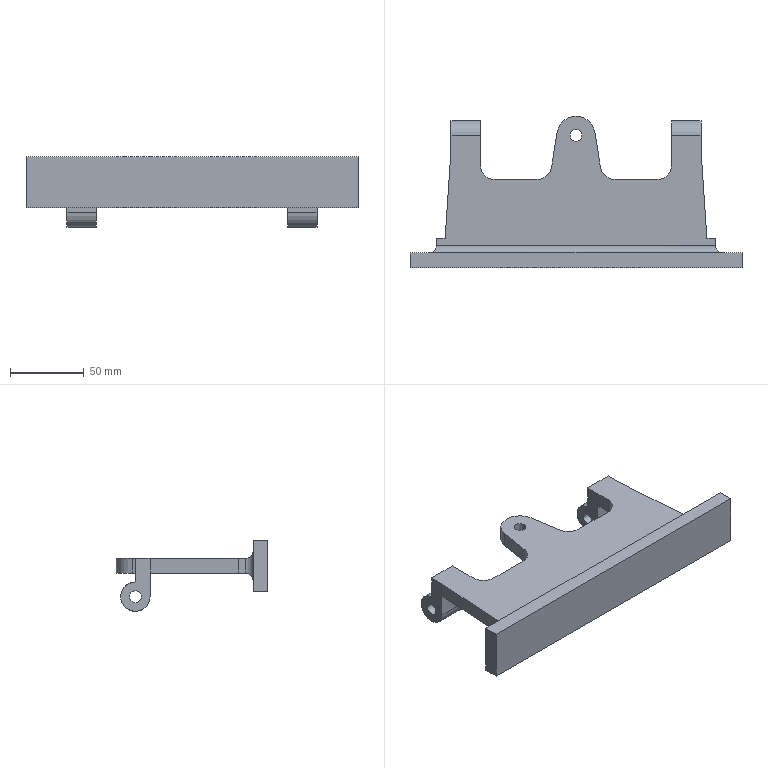Part | SolidWorks | features ICE 2, Extrusion 1, Fillet 1, MirrorPattern 1 | 1 solid | 44 faces | box 225.743 x 103 x 48.082 mm | volume 208388 mm3 | plane 26 | cylinder 18 | commonest cylinder face diameters 20 x7 8 x6 10 x4 26 x1
STEP:
#1=CARTESIAN_POINT('',(85.,-4.,-16.));
#2=VERTEX_POINT('',#1);
#3=CARTESIAN_POINT('',(85.,4.,-16.));
#4=VERTEX_POINT('',#3);
#5=CARTESIAN_POINT('',(85.,0.,-16.));
#6=DIRECTION('',(1.,0.,0.));
#7=DIRECTION('',(0.,1.,0.));
#8=AXIS2_PLACEMENT_3D('',#5,#6,#7);
#9=CIRCLE('',#8,4.);
#10=EDGE_CURVE('',#2,#4,#9,.T.);
#11=ORIENTED_EDGE('',*,*,#10,.T.);
#12=CARTESIAN_POINT('',(65.,4.,-16.));
#13=VERTEX_POINT('',#12);
#14=CARTESIAN_POINT('',(85.,4.,-16.));
#15=DIRECTION('',(-1.,0.,0.));
#16=VECTOR('',#15,1000.);
#17=LINE('',#14,#16);
#18=EDGE_CURVE('',#4,#13,#17,.T.);
#19=ORIENTED_EDGE('',*,*,#18,.T.);
#20=CARTESIAN_POINT('',(65.,-4.,-16.));
#21=VERTEX_POINT('',#20);
#22=CARTESIAN_POINT('',(65.,0.,-16.));
#23=DIRECTION('',(1.,0.,0.));
#24=DIRECTION('',(0.,1.,0.));
#25=AXIS2_PLACEMENT_3D('',#22,#23,#24);
#26=CIRCLE('',#25,4.);
#27=EDGE_CURVE('',#21,#13,#26,.T.);
#28=ORIENTED_EDGE('',*,*,#27,.F.);
#29=CARTESIAN_POINT('',(85.,-4.,-16.));
#30=DIRECTION('',(-1.,0.,0.));
#31=VECTOR('',#30,1000.);
#32=LINE('',#29,#31);
#33=EDGE_CURVE('',#2,#21,#32,.T.);
#34=ORIENTED_EDGE('',*,*,#33,.F.);
#35=EDGE_LOOP('',(#11,#19,#28,#34));
#36=FACE_OUTER_BOUND('',#35,.T.);
#37=CARTESIAN_POINT('',(85.,0.,-16.));
#38=DIRECTION('',(-1.,0.,0.));
#39=DIRECTION('',(0.,-1.,0.));
#40=AXIS2_PLACEMENT_3D('',#37,#38,#39);
#41=CYLINDRICAL_SURFACE('',#40,4.);
#42=ADVANCED_FACE('',(#36),#41,.F.);
#43=CARTESIAN_POINT('',(-85.,-4.,-16.));
#44=VERTEX_POINT('',#43);
#45=CARTESIAN_POINT('',(-85.,4.,-16.));
#46=VERTEX_POINT('',#45);
#47=CARTESIAN_POINT('',(-85.,0.,-16.));
#48=DIRECTION('',(1.,0.,0.));
#49=DIRECTION('',(0.,1.,0.));
#50=AXIS2_PLACEMENT_3D('',#47,#48,#49);
#51=CIRCLE('',#50,4.);
#52=EDGE_CURVE('',#44,#46,#51,.T.);
#53=ORIENTED_EDGE('',*,*,#52,.F.);
#54=CARTESIAN_POINT('',(-65.,-4.,-16.));
#55=VERTEX_POINT('',#54);
#56=CARTESIAN_POINT('',(-85.,-4.,-16.));
#57=DIRECTION('',(1.,0.,0.));
#58=VECTOR('',#57,1000.);
#59=LINE('',#56,#58);
#60=EDGE_CURVE('',#44,#55,#59,.T.);
#61=ORIENTED_EDGE('',*,*,#60,.T.);
#62=CARTESIAN_POINT('',(-65.,4.,-16.));
#63=VERTEX_POINT('',#62);
#64=CARTESIAN_POINT('',(-65.,0.,-16.));
#65=DIRECTION('',(1.,0.,0.));
#66=DIRECTION('',(0.,1.,0.));
#67=AXIS2_PLACEMENT_3D('',#64,#65,#66);
#68=CIRCLE('',#67,4.);
#69=EDGE_CURVE('',#55,#63,#68,.T.);
#70=ORIENTED_EDGE('',*,*,#69,.T.);
#71=CARTESIAN_POINT('',(-85.,4.,-16.));
#72=DIRECTION('',(1.,0.,0.));
#73=VECTOR('',#72,1000.);
#74=LINE('',#71,#73);
#75=EDGE_CURVE('',#46,#63,#74,.T.);
#76=ORIENTED_EDGE('',*,*,#75,.F.);
#77=EDGE_LOOP('',(#53,#61,#70,#76));
#78=FACE_OUTER_BOUND('',#77,.T.);
#79=CARTESIAN_POINT('',(-85.,0.,-16.));
#80=DIRECTION('',(1.,0.,0.));
#81=DIRECTION('',(0.,1.,0.));
#82=AXIS2_PLACEMENT_3D('',#79,#80,#81);
#83=CYLINDRICAL_SURFACE('',#82,4.);
#84=ADVANCED_FACE('',(#78),#83,.F.);
#85=CARTESIAN_POINT('',(-85.,-10.,-16.));
#86=VERTEX_POINT('',#85);
#87=CARTESIAN_POINT('',(-85.,10.,-16.));
#88=VERTEX_POINT('',#87);
#89=CARTESIAN_POINT('',(-85.,0.,-16.));
#90=DIRECTION('',(1.,0.,0.));
#91=DIRECTION('',(0.,1.,0.));
#92=AXIS2_PLACEMENT_3D('',#89,#90,#91);
#93=CIRCLE('',#92,10.);
#94=EDGE_CURVE('',#86,#88,#93,.T.);
#95=ORIENTED_EDGE('',*,*,#94,.T.);
#96=CARTESIAN_POINT('',(-65.,10.,-16.));
#97=VERTEX_POINT('',#96);
#98=CARTESIAN_POINT('',(-85.,10.,-16.));
#99=DIRECTION('',(1.,0.,0.));
#100=VECTOR('',#99,1000.);
#101=LINE('',#98,#100);
#102=EDGE_CURVE('',#88,#97,#101,.T.);
#103=ORIENTED_EDGE('',*,*,#102,.T.);
#104=CARTESIAN_POINT('',(-65.,-10.,-16.));
#105=VERTEX_POINT('',#104);
#106=CARTESIAN_POINT('',(-65.,0.,-16.));
#107=DIRECTION('',(1.,0.,0.));
#108=DIRECTION('',(0.,1.,0.));
#109=AXIS2_PLACEMENT_3D('',#106,#107,#108);
#110=CIRCLE('',#109,10.);
#111=EDGE_CURVE('',#105,#97,#110,.T.);
#112=ORIENTED_EDGE('',*,*,#111,.F.);
#113=CARTESIAN_POINT('',(-85.,-10.,-16.));
#114=DIRECTION('',(1.,0.,0.));
#115=VECTOR('',#114,1000.);
#116=LINE('',#113,#115);
#117=EDGE_CURVE('',#86,#105,#116,.T.);
#118=ORIENTED_EDGE('',*,*,#117,.F.);
#119=EDGE_LOOP('',(#95,#103,#112,#118));
#120=FACE_OUTER_BOUND('',#119,.T.);
#121=CARTESIAN_POINT('',(-85.,0.,-16.));
#122=DIRECTION('',(1.,0.,0.));
#123=DIRECTION('',(0.,1.,0.));
#124=AXIS2_PLACEMENT_3D('',#121,#122,#123);
#125=CYLINDRICAL_SURFACE('',#124,10.);
#126=ADVANCED_FACE('',(#120),#125,.T.);
#127=CARTESIAN_POINT('',(-4.,0.,10.));
#128=VERTEX_POINT('',#127);
#129=CARTESIAN_POINT('',(4.,0.,10.));
#130=VERTEX_POINT('',#129);
#131=CARTESIAN_POINT('',(0.,0.,10.));
#132=DIRECTION('',(0.,0.,1.));
#133=DIRECTION('',(1.,0.,0.));
#134=AXIS2_PLACEMENT_3D('',#131,#132,#133);
#135=CIRCLE('',#134,4.);
#136=EDGE_CURVE('',#128,#130,#135,.T.);
#137=ORIENTED_EDGE('',*,*,#136,.T.);
#138=CARTESIAN_POINT('',(4.,0.,0.));
#139=VERTEX_POINT('',#138);
#140=CARTESIAN_POINT('',(4.,0.,10.));
#141=DIRECTION('',(0.,0.,-1.));
#142=VECTOR('',#141,1000.);
#143=LINE('',#140,#142);
#144=EDGE_CURVE('',#130,#139,#143,.T.);
#145=ORIENTED_EDGE('',*,*,#144,.T.);
#146=CARTESIAN_POINT('',(-4.,0.,0.));
#147=VERTEX_POINT('',#146);
#148=CARTESIAN_POINT('',(0.,0.,0.));
#149=DIRECTION('',(0.,0.,1.));
#150=DIRECTION('',(1.,0.,0.));
#151=AXIS2_PLACEMENT_3D('',#148,#149,#150);
#152=CIRCLE('',#151,4.);
#153=EDGE_CURVE('',#147,#139,#152,.T.);
#154=ORIENTED_EDGE('',*,*,#153,.F.);
#155=CARTESIAN_POINT('',(-4.,0.,10.));
#156=DIRECTION('',(0.,0.,-1.));
#157=VECTOR('',#156,1000.);
#158=LINE('',#155,#157);
#159=EDGE_CURVE('',#128,#147,#158,.T.);
#160=ORIENTED_EDGE('',*,*,#159,.F.);
#161=EDGE_LOOP('',(#137,#145,#154,#160));
#162=FACE_OUTER_BOUND('',#161,.T.);
#163=CARTESIAN_POINT('',(0.,0.,10.));
#164=DIRECTION('',(0.,0.,-1.));
#165=DIRECTION('',(-1.,0.,0.));
#166=AXIS2_PLACEMENT_3D('',#163,#164,#165);
#167=CYLINDRICAL_SURFACE('',#166,4.);
#168=ADVANCED_FACE('',(#162),#167,.F.);
#169=CARTESIAN_POINT('',(-95.,-70.,10.));
#170=VERTEX_POINT('',#169);
#171=CARTESIAN_POINT('',(-95.,-75.,10.));
#172=VERTEX_POINT('',#171);
#173=CARTESIAN_POINT('',(-95.,-80.,10.));
#174=DIRECTION('',(0.,-1.,0.));
#175=VECTOR('',#174,1000.);
#176=LINE('',#173,#175);
#177=EDGE_CURVE('',#170,#172,#176,.T.);
#178=ORIENTED_EDGE('',*,*,#177,.T.);
#179=CARTESIAN_POINT('',(95.,-75.,10.));
#180=VERTEX_POINT('',#179);
#181=CARTESIAN_POINT('',(95.,-75.,10.));
#182=DIRECTION('',(1.,0.,0.));
#183=VECTOR('',#182,1000.);
#184=LINE('',#181,#183);
#185=EDGE_CURVE('',#172,#180,#184,.T.);
#186=ORIENTED_EDGE('',*,*,#185,.T.);
#187=CARTESIAN_POINT('',(95.,-70.,10.));
#188=VERTEX_POINT('',#187);
#189=CARTESIAN_POINT('',(95.,-80.,10.));
#190=DIRECTION('',(0.,1.,0.));
#191=VECTOR('',#190,1000.);
#192=LINE('',#189,#191);
#193=EDGE_CURVE('',#180,#188,#192,.T.);
#194=ORIENTED_EDGE('',*,*,#193,.T.);
#195=CARTESIAN_POINT('',(89.,-70.,10.));
#196=VERTEX_POINT('',#195);
#197=CARTESIAN_POINT('',(95.,-70.,10.));
#198=DIRECTION('',(-1.,0.,0.));
#199=VECTOR('',#198,1000.);
#200=LINE('',#197,#199);
#201=EDGE_CURVE('',#188,#196,#200,.T.);
#202=ORIENTED_EDGE('',*,*,#201,.T.);
#203=CARTESIAN_POINT('',(85.,-10.,10.));
#204=VERTEX_POINT('',#203);
#205=CARTESIAN_POINT('',(85.,-10.,10.));
#206=DIRECTION('',(-0.06652,0.9978,0.));
#207=VECTOR('',#206,1000.);
#208=LINE('',#205,#207);
#209=EDGE_CURVE('',#196,#204,#208,.T.);
#210=ORIENTED_EDGE('',*,*,#209,.T.);
#211=CARTESIAN_POINT('',(85.,0.,10.));
#212=VERTEX_POINT('',#211);
#213=CARTESIAN_POINT('',(85.,0.,10.));
#214=DIRECTION('',(0.,-1.,0.));
#215=VECTOR('',#214,1000.);
#216=LINE('',#213,#215);
#217=EDGE_CURVE('',#212,#204,#216,.T.);
#218=ORIENTED_EDGE('',*,*,#217,.F.);
#219=CARTESIAN_POINT('',(65.,0.,10.));
#220=VERTEX_POINT('',#219);
#221=CARTESIAN_POINT('',(85.,0.,10.));
#222=DIRECTION('',(-1.,0.,0.));
#223=VECTOR('',#222,1000.);
#224=LINE('',#221,#223);
#225=EDGE_CURVE('',#212,#220,#224,.T.);
#226=ORIENTED_EDGE('',*,*,#225,.T.);
#227=CARTESIAN_POINT('',(65.,-20.,10.));
#228=VERTEX_POINT('',#227);
#229=CARTESIAN_POINT('',(65.,-10.,10.));
#230=DIRECTION('',(0.,-1.,0.));
#231=VECTOR('',#230,1000.);
#232=LINE('',#229,#231);
#233=EDGE_CURVE('',#220,#228,#232,.T.);
#234=ORIENTED_EDGE('',*,*,#233,.T.);
#235=CARTESIAN_POINT('',(55.,-30.,10.));
#236=VERTEX_POINT('',#235);
#237=CARTESIAN_POINT('',(55.,-20.,10.));
#238=DIRECTION('',(0.,0.,-1.));
#239=DIRECTION('',(-1.,0.,0.));
#240=AXIS2_PLACEMENT_3D('',#237,#238,#239);
#241=CIRCLE('',#240,10.);
#242=EDGE_CURVE('',#228,#236,#241,.T.);
#243=ORIENTED_EDGE('',*,*,#242,.T.);
#244=CARTESIAN_POINT('',(26.518,-30.,10.));
#245=VERTEX_POINT('',#244);
#246=CARTESIAN_POINT('',(26.518,-30.,10.));
#247=DIRECTION('',(-1.,0.,0.));
#248=VECTOR('',#247,1000.);
#249=LINE('',#246,#248);
#250=EDGE_CURVE('',#236,#245,#249,.T.);
#251=ORIENTED_EDGE('',*,*,#250,.T.);
#252=CARTESIAN_POINT('',(16.645,-21.59,10.));
#253=VERTEX_POINT('',#252);
#254=CARTESIAN_POINT('',(26.518,-20.,10.));
#255=DIRECTION('',(0.,0.,-1.));
#256=DIRECTION('',(1.,0.,0.));
#257=AXIS2_PLACEMENT_3D('',#254,#255,#256);
#258=CIRCLE('',#257,10.);
#259=EDGE_CURVE('',#245,#253,#258,.T.);
#260=ORIENTED_EDGE('',*,*,#259,.T.);
#261=CARTESIAN_POINT('',(12.835,2.067,10.));
#262=VERTEX_POINT('',#261);
#263=CARTESIAN_POINT('',(12.835,2.067,10.));
#264=DIRECTION('',(-0.159,0.9873,0.));
#265=VECTOR('',#264,1000.);
#266=LINE('',#263,#265);
#267=EDGE_CURVE('',#253,#262,#266,.T.);
#268=ORIENTED_EDGE('',*,*,#267,.T.);
#269=CARTESIAN_POINT('',(-12.835,2.067,10.));
#270=VERTEX_POINT('',#269);
#271=CARTESIAN_POINT('',(0.,0.,10.));
#272=DIRECTION('',(0.,0.,1.));
#273=DIRECTION('',(1.,0.,0.));
#274=AXIS2_PLACEMENT_3D('',#271,#272,#273);
#275=CIRCLE('',#274,13.);
#276=EDGE_CURVE('',#262,#270,#275,.T.);
#277=ORIENTED_EDGE('',*,*,#276,.T.);
#278=CARTESIAN_POINT('',(-16.645,-21.59,10.));
#279=VERTEX_POINT('',#278);
#280=CARTESIAN_POINT('',(-12.835,2.067,10.));
#281=DIRECTION('',(-0.159,-0.9873,0.));
#282=VECTOR('',#281,1000.);
#283=LINE('',#280,#282);
#284=EDGE_CURVE('',#270,#279,#283,.T.);
#285=ORIENTED_EDGE('',*,*,#284,.T.);
#286=CARTESIAN_POINT('',(-26.518,-30.,10.));
#287=VERTEX_POINT('',#286);
#288=CARTESIAN_POINT('',(-26.518,-20.,10.));
#289=DIRECTION('',(0.,0.,-1.));
#290=DIRECTION('',(-1.,0.,0.));
#291=AXIS2_PLACEMENT_3D('',#288,#289,#290);
#292=CIRCLE('',#291,10.);
#293=EDGE_CURVE('',#279,#287,#292,.T.);
#294=ORIENTED_EDGE('',*,*,#293,.T.);
#295=CARTESIAN_POINT('',(-55.,-30.,10.));
#296=VERTEX_POINT('',#295);
#297=CARTESIAN_POINT('',(-55.,-30.,10.));
#298=DIRECTION('',(-1.,0.,0.));
#299=VECTOR('',#298,1000.);
#300=LINE('',#297,#299);
#301=EDGE_CURVE('',#287,#296,#300,.T.);
#302=ORIENTED_EDGE('',*,*,#301,.T.);
#303=CARTESIAN_POINT('',(-65.,-20.,10.));
#304=VERTEX_POINT('',#303);
#305=CARTESIAN_POINT('',(-55.,-20.,10.));
#306=DIRECTION('',(0.,0.,-1.));
#307=DIRECTION('',(1.,0.,0.));
#308=AXIS2_PLACEMENT_3D('',#305,#306,#307);
#309=CIRCLE('',#308,10.);
#310=EDGE_CURVE('',#296,#304,#309,.T.);
#311=ORIENTED_EDGE('',*,*,#310,.T.);
#312=CARTESIAN_POINT('',(-65.,0.,10.));
#313=VERTEX_POINT('',#312);
#314=CARTESIAN_POINT('',(-65.,-10.,10.));
#315=DIRECTION('',(0.,1.,0.));
#316=VECTOR('',#315,1000.);
#317=LINE('',#314,#316);
#318=EDGE_CURVE('',#304,#313,#317,.T.);
#319=ORIENTED_EDGE('',*,*,#318,.T.);
#320=CARTESIAN_POINT('',(-85.,0.,10.));
#321=VERTEX_POINT('',#320);
#322=CARTESIAN_POINT('',(-85.,0.,10.));
#323=DIRECTION('',(1.,0.,0.));
#324=VECTOR('',#323,1000.);
#325=LINE('',#322,#324);
#326=EDGE_CURVE('',#321,#313,#325,.T.);
#327=ORIENTED_EDGE('',*,*,#326,.F.);
#328=CARTESIAN_POINT('',(-85.,-10.,10.));
#329=VERTEX_POINT('',#328);
#330=CARTESIAN_POINT('',(-85.,0.,10.));
#331=DIRECTION('',(0.,-1.,0.));
#332=VECTOR('',#331,1000.);
#333=LINE('',#330,#332);
#334=EDGE_CURVE('',#321,#329,#333,.T.);
#335=ORIENTED_EDGE('',*,*,#334,.T.);
#336=CARTESIAN_POINT('',(-89.,-70.,10.));
#337=VERTEX_POINT('',#336);
#338=CARTESIAN_POINT('',(-85.,-10.,10.));
#339=DIRECTION('',(-0.06652,-0.9978,0.));
#340=VECTOR('',#339,1000.);
#341=LINE('',#338,#340);
#342=EDGE_CURVE('',#329,#337,#341,.T.);
#343=ORIENTED_EDGE('',*,*,#342,.T.);
#344=CARTESIAN_POINT('',(-95.,-70.,10.));
#345=DIRECTION('',(-1.,0.,0.));
#346=VECTOR('',#345,1000.);
#347=LINE('',#344,#346);
#348=EDGE_CURVE('',#337,#170,#347,.T.);
#349=ORIENTED_EDGE('',*,*,#348,.T.);
#350=EDGE_LOOP('',(#178,#186,#194,#202,#210,#218,#226,#234,#243,#251,#260,#268,#277,#285,#294,#302,#311,#319,#327,#335,#343,#349));
#351=FACE_OUTER_BOUND('',#350,.T.);
#352=ORIENTED_EDGE('',*,*,#136,.F.);
#353=CARTESIAN_POINT('',(0.,0.,10.));
#354=DIRECTION('',(0.,0.,1.));
#355=DIRECTION('',(1.,0.,0.));
#356=AXIS2_PLACEMENT_3D('',#353,#354,#355);
#357=CIRCLE('',#356,4.);
#358=EDGE_CURVE('',#130,#128,#357,.T.);
#359=ORIENTED_EDGE('',*,*,#358,.F.);
#360=EDGE_LOOP('',(#352,#359));
#361=FACE_BOUND('',#360,.T.);
#362=CARTESIAN_POINT('',(55.,-20.,10.));
#363=DIRECTION('',(0.,0.,-1.));
#364=DIRECTION('',(-1.,0.,0.));
#365=AXIS2_PLACEMENT_3D('',#362,#363,#364);
#366=PLANE('',#365);
#367=ADVANCED_FACE('',(#351,#361),#366,.F.);
#368=CARTESIAN_POINT('',(95.,-75.,0.));
#369=VERTEX_POINT('',#368);
#370=CARTESIAN_POINT('',(95.,-70.,0.));
#371=VERTEX_POINT('',#370);
#372=CARTESIAN_POINT('',(95.,-80.,0.));
#373=DIRECTION('',(0.,1.,0.));
#374=VECTOR('',#373,1000.);
#375=LINE('',#372,#374);
#376=EDGE_CURVE('',#369,#371,#375,.T.);
#377=ORIENTED_EDGE('',*,*,#376,.F.);
#378=CARTESIAN_POINT('',(-95.,-75.,0.));
#379=VERTEX_POINT('',#378);
#380=CARTESIAN_POINT('',(55.,-75.,0.));
#381=DIRECTION('',(-1.,0.,0.));
#382=VECTOR('',#381,1000.);
#383=LINE('',#380,#382);
#384=EDGE_CURVE('',#369,#379,#383,.T.);
#385=ORIENTED_EDGE('',*,*,#384,.T.);
#386=CARTESIAN_POINT('',(-95.,-70.,0.));
#387=VERTEX_POINT('',#386);
#388=CARTESIAN_POINT('',(-95.,-80.,0.));
#389=DIRECTION('',(0.,-1.,0.));
#390=VECTOR('',#389,1000.);
#391=LINE('',#388,#390);
#392=EDGE_CURVE('',#387,#379,#391,.T.);
#393=ORIENTED_EDGE('',*,*,#392,.F.);
#394=CARTESIAN_POINT('',(-89.,-70.,0.));
#395=VERTEX_POINT('',#394);
#396=CARTESIAN_POINT('',(-95.,-70.,0.));
#397=DIRECTION('',(-1.,0.,0.));
#398=VECTOR('',#397,1000.);
#399=LINE('',#396,#398);
#400=EDGE_CURVE('',#395,#387,#399,.T.);
#401=ORIENTED_EDGE('',*,*,#400,.F.);
#402=CARTESIAN_POINT('',(-85.,-10.,0.));
#403=VERTEX_POINT('',#402);
#404=CARTESIAN_POINT('',(-85.,-10.,0.));
#405=DIRECTION('',(-0.06652,-0.9978,0.));
#406=VECTOR('',#405,1000.);
#407=LINE('',#404,#406);
#408=EDGE_CURVE('',#403,#395,#407,.T.);
#409=ORIENTED_EDGE('',*,*,#408,.F.);
#410=CARTESIAN_POINT('',(-65.,-10.,0.));
#411=VERTEX_POINT('',#410);
#412=CARTESIAN_POINT('',(-65.,-10.,0.));
#413=DIRECTION('',(-1.,0.,0.));
#414=VECTOR('',#413,1000.);
#415=LINE('',#412,#414);
#416=EDGE_CURVE('',#411,#403,#415,.T.);
#417=ORIENTED_EDGE('',*,*,#416,.F.);
#418=CARTESIAN_POINT('',(-65.,-20.,0.));
#419=VERTEX_POINT('',#418);
#420=CARTESIAN_POINT('',(-65.,-10.,0.));
#421=DIRECTION('',(0.,1.,0.));
#422=VECTOR('',#421,1000.);
#423=LINE('',#420,#422);
#424=EDGE_CURVE('',#419,#411,#423,.T.);
#425=ORIENTED_EDGE('',*,*,#424,.F.);
#426=CARTESIAN_POINT('',(-55.,-30.,0.));
#427=VERTEX_POINT('',#426);
#428=CARTESIAN_POINT('',(-55.,-20.,0.));
#429=DIRECTION('',(0.,0.,-1.));
#430=DIRECTION('',(1.,0.,0.));
#431=AXIS2_PLACEMENT_3D('',#428,#429,#430);
#432=CIRCLE('',#431,10.);
#433=EDGE_CURVE('',#427,#419,#432,.T.);
#434=ORIENTED_EDGE('',*,*,#433,.F.);
#435=CARTESIAN_POINT('',(-26.518,-30.,0.));
#436=VERTEX_POINT('',#435);
#437=CARTESIAN_POINT('',(-55.,-30.,0.));
#438=DIRECTION('',(-1.,0.,0.));
#439=VECTOR('',#438,1000.);
#440=LINE('',#437,#439);
#441=EDGE_CURVE('',#436,#427,#440,.T.);
#442=ORIENTED_EDGE('',*,*,#441,.F.);
#443=CARTESIAN_POINT('',(-16.645,-21.59,0.));
#444=VERTEX_POINT('',#443);
#445=CARTESIAN_POINT('',(-26.518,-20.,0.));
#446=DIRECTION('',(0.,0.,-1.));
#447=DIRECTION('',(-1.,0.,0.));
#448=AXIS2_PLACEMENT_3D('',#445,#446,#447);
#449=CIRCLE('',#448,10.);
#450=EDGE_CURVE('',#444,#436,#449,.T.);
#451=ORIENTED_EDGE('',*,*,#450,.F.);
#452=CARTESIAN_POINT('',(-12.835,2.067,0.));
#453=VERTEX_POINT('',#452);
#454=CARTESIAN_POINT('',(-12.835,2.067,0.));
#455=DIRECTION('',(-0.159,-0.9873,0.));
#456=VECTOR('',#455,1000.);
#457=LINE('',#454,#456);
#458=EDGE_CURVE('',#453,#444,#457,.T.);
#459=ORIENTED_EDGE('',*,*,#458,.F.);
#460=CARTESIAN_POINT('',(12.835,2.067,0.));
#461=VERTEX_POINT('',#460);
#462=CARTESIAN_POINT('',(0.,0.,0.));
#463=DIRECTION('',(0.,0.,1.));
#464=DIRECTION('',(1.,0.,0.));
#465=AXIS2_PLACEMENT_3D('',#462,#463,#464);
#466=CIRCLE('',#465,13.);
#467=EDGE_CURVE('',#461,#453,#466,.T.);
#468=ORIENTED_EDGE('',*,*,#467,.F.);
#469=CARTESIAN_POINT('',(16.645,-21.59,0.));
#470=VERTEX_POINT('',#469);
#471=CARTESIAN_POINT('',(12.835,2.067,0.));
#472=DIRECTION('',(-0.159,0.9873,0.));
#473=VECTOR('',#472,1000.);
#474=LINE('',#471,#473);
#475=EDGE_CURVE('',#470,#461,#474,.T.);
#476=ORIENTED_EDGE('',*,*,#475,.F.);
#477=CARTESIAN_POINT('',(26.518,-30.,0.));
#478=VERTEX_POINT('',#477);
#479=CARTESIAN_POINT('',(26.518,-20.,0.));
#480=DIRECTION('',(0.,0.,-1.));
#481=DIRECTION('',(1.,0.,0.));
#482=AXIS2_PLACEMENT_3D('',#479,#480,#481);
#483=CIRCLE('',#482,10.);
#484=EDGE_CURVE('',#478,#470,#483,.T.);
#485=ORIENTED_EDGE('',*,*,#484,.F.);
#486=CARTESIAN_POINT('',(55.,-30.,0.));
#487=VERTEX_POINT('',#486);
#488=CARTESIAN_POINT('',(26.518,-30.,0.));
#489=DIRECTION('',(-1.,0.,0.));
#490=VECTOR('',#489,1000.);
#491=LINE('',#488,#490);
#492=EDGE_CURVE('',#487,#478,#491,.T.);
#493=ORIENTED_EDGE('',*,*,#492,.F.);
#494=CARTESIAN_POINT('',(65.,-20.,0.));
#495=VERTEX_POINT('',#494);
#496=CARTESIAN_POINT('',(55.,-20.,0.));
#497=DIRECTION('',(0.,0.,-1.));
#498=DIRECTION('',(-1.,0.,0.));
#499=AXIS2_PLACEMENT_3D('',#496,#497,#498);
#500=CIRCLE('',#499,10.);
#501=EDGE_CURVE('',#495,#487,#500,.T.);
#502=ORIENTED_EDGE('',*,*,#501,.F.);
#503=CARTESIAN_POINT('',(65.,-10.,0.));
#504=VERTEX_POINT('',#503);
#505=CARTESIAN_POINT('',(65.,-10.,0.));
#506=DIRECTION('',(0.,-1.,0.));
#507=VECTOR('',#506,1000.);
#508=LINE('',#505,#507);
#509=EDGE_CURVE('',#504,#495,#508,.T.);
#510=ORIENTED_EDGE('',*,*,#509,.F.);
#511=CARTESIAN_POINT('',(85.,-10.,0.));
#512=VERTEX_POINT('',#511);
#513=CARTESIAN_POINT('',(65.,-10.,0.));
#514=DIRECTION('',(-1.,0.,0.));
#515=VECTOR('',#514,1000.);
#516=LINE('',#513,#515);
#517=EDGE_CURVE('',#512,#504,#516,.T.);
#518=ORIENTED_EDGE('',*,*,#517,.F.);
#519=CARTESIAN_POINT('',(89.,-70.,0.));
#520=VERTEX_POINT('',#519);
#521=CARTESIAN_POINT('',(85.,-10.,0.));
#522=DIRECTION('',(-0.06652,0.9978,0.));
#523=VECTOR('',#522,1000.);
#524=LINE('',#521,#523);
#525=EDGE_CURVE('',#520,#512,#524,.T.);
#526=ORIENTED_EDGE('',*,*,#525,.F.);
#527=CARTESIAN_POINT('',(95.,-70.,0.));
#528=DIRECTION('',(-1.,0.,0.));
#529=VECTOR('',#528,1000.);
#530=LINE('',#527,#529);
#531=EDGE_CURVE('',#371,#520,#530,.T.);
#532=ORIENTED_EDGE('',*,*,#531,.F.);
#533=EDGE_LOOP('',(#377,#385,#393,#401,#409,#417,#425,#434,#442,#451,#459,#468,#476,#485,#493,#502,#510,#518,#526,#532));
#534=FACE_OUTER_BOUND('',#533,.T.);
#535=ORIENTED_EDGE('',*,*,#153,.T.);
#536=CARTESIAN_POINT('',(0.,0.,0.));
#537=DIRECTION('',(0.,0.,1.));
#538=DIRECTION('',(1.,0.,0.));
#539=AXIS2_PLACEMENT_3D('',#536,#537,#538);
#540=CIRCLE('',#539,4.);
#541=EDGE_CURVE('',#139,#147,#540,.T.);
#542=ORIENTED_EDGE('',*,*,#541,.T.);
#543=EDGE_LOOP('',(#535,#542));
#544=FACE_BOUND('',#543,.T.);
#545=CARTESIAN_POINT('',(55.,-20.,0.));
#546=DIRECTION('',(0.,0.,-1.));
#547=DIRECTION('',(-1.,0.,0.));
#548=AXIS2_PLACEMENT_3D('',#545,#546,#547);
#549=PLANE('',#548);
#550=ADVANCED_FACE('',(#534,#544),#549,.T.);
#551=ORIENTED_EDGE('',*,*,#531,.T.);
#552=CARTESIAN_POINT('',(89.,-70.,10.));
#553=DIRECTION('',(0.,0.,-1.));
#554=VECTOR('',#553,1000.);
#555=LINE('',#552,#554);
#556=EDGE_CURVE('',#196,#520,#555,.T.);
#557=ORIENTED_EDGE('',*,*,#556,.F.);
#558=ORIENTED_EDGE('',*,*,#201,.F.);
#559=CARTESIAN_POINT('',(95.,-70.,10.));
#560=DIRECTION('',(0.,0.,-1.));
#561=VECTOR('',#560,1000.);
#562=LINE('',#559,#561);
#563=EDGE_CURVE('',#188,#371,#562,.T.);
#564=ORIENTED_EDGE('',*,*,#563,.T.);
#565=EDGE_LOOP('',(#551,#557,#558,#564));
#566=FACE_OUTER_BOUND('',#565,.T.);
#567=CARTESIAN_POINT('',(95.,-70.,10.));
#568=DIRECTION('',(0.,-1.,0.));
#569=DIRECTION('',(1.,0.,0.));
#570=AXIS2_PLACEMENT_3D('',#567,#568,#569);
#571=PLANE('',#570);
#572=ADVANCED_FACE('',(#566),#571,.F.);
#573=ORIENTED_EDGE('',*,*,#525,.T.);
#574=CARTESIAN_POINT('',(85.,-10.,10.));
#575=DIRECTION('',(0.,0.,-1.));
#576=VECTOR('',#575,1000.);
#577=LINE('',#574,#576);
#578=EDGE_CURVE('',#204,#512,#577,.T.);
#579=ORIENTED_EDGE('',*,*,#578,.F.);
#580=ORIENTED_EDGE('',*,*,#209,.F.);
#581=ORIENTED_EDGE('',*,*,#556,.T.);
#582=EDGE_LOOP('',(#573,#579,#580,#581));
#583=FACE_OUTER_BOUND('',#582,.T.);
#584=CARTESIAN_POINT('',(85.,-10.,10.));
#585=DIRECTION('',(-0.9978,-0.06652,0.));
#586=DIRECTION('',(0.06652,-0.9978,0.));
#587=AXIS2_PLACEMENT_3D('',#584,#585,#586);
#588=PLANE('',#587);
#589=ADVANCED_FACE('',(#583),#588,.F.);
#590=ORIENTED_EDGE('',*,*,#509,.T.);
#591=CARTESIAN_POINT('',(65.,-20.,10.));
#592=DIRECTION('',(0.,0.,-1.));
#593=VECTOR('',#592,1000.);
#594=LINE('',#591,#593);
#595=EDGE_CURVE('',#228,#495,#594,.T.);
#596=ORIENTED_EDGE('',*,*,#595,.F.);
#597=ORIENTED_EDGE('',*,*,#233,.F.);
#598=CARTESIAN_POINT('',(65.,0.,-6.));
#599=VERTEX_POINT('',#598);
#600=CARTESIAN_POINT('',(65.,0.,-6.));
#601=DIRECTION('',(0.,0.,1.));
#602=VECTOR('',#601,1000.);
#603=LINE('',#600,#602);
#604=EDGE_CURVE('',#599,#220,#603,.T.);
#605=ORIENTED_EDGE('',*,*,#604,.F.);
#606=CARTESIAN_POINT('',(65.,-10.,-16.));
#607=VERTEX_POINT('',#606);
#608=CARTESIAN_POINT('',(65.,0.,-16.));
#609=DIRECTION('',(1.,0.,0.));
#610=DIRECTION('',(0.,1.,0.));
#611=AXIS2_PLACEMENT_3D('',#608,#609,#610);
#612=CIRCLE('',#611,10.);
#613=EDGE_CURVE('',#607,#599,#612,.T.);
#614=ORIENTED_EDGE('',*,*,#613,.F.);
#615=CARTESIAN_POINT('',(65.,-10.,10.));
#616=DIRECTION('',(0.,0.,-1.));
#617=VECTOR('',#616,1000.);
#618=LINE('',#615,#617);
#619=EDGE_CURVE('',#504,#607,#618,.T.);
#620=ORIENTED_EDGE('',*,*,#619,.F.);
#621=EDGE_LOOP('',(#590,#596,#597,#605,#614,#620));
#622=FACE_OUTER_BOUND('',#621,.T.);
#623=ORIENTED_EDGE('',*,*,#27,.T.);
#624=CARTESIAN_POINT('',(65.,0.,-16.));
#625=DIRECTION('',(1.,0.,0.));
#626=DIRECTION('',(0.,1.,0.));
#627=AXIS2_PLACEMENT_3D('',#624,#625,#626);
#628=CIRCLE('',#627,4.);
#629=EDGE_CURVE('',#13,#21,#628,.T.);
#630=ORIENTED_EDGE('',*,*,#629,.T.);
#631=EDGE_LOOP('',(#623,#630));
#632=FACE_BOUND('',#631,.T.);
#633=CARTESIAN_POINT('',(65.,-10.,10.));
#634=DIRECTION('',(1.,0.,0.));
#635=DIRECTION('',(0.,0.,-1.));
#636=AXIS2_PLACEMENT_3D('',#633,#634,#635);
#637=PLANE('',#636);
#638=ADVANCED_FACE('',(#622,#632),#637,.F.);
#639=ORIENTED_EDGE('',*,*,#501,.T.);
#640=CARTESIAN_POINT('',(55.,-30.,10.));
#641=DIRECTION('',(0.,0.,-1.));
#642=VECTOR('',#641,1000.);
#643=LINE('',#640,#642);
#644=EDGE_CURVE('',#236,#487,#643,.T.);
#645=ORIENTED_EDGE('',*,*,#644,.F.);
#646=ORIENTED_EDGE('',*,*,#242,.F.);
#647=ORIENTED_EDGE('',*,*,#595,.T.);
#648=EDGE_LOOP('',(#639,#645,#646,#647));
#649=FACE_OUTER_BOUND('',#648,.T.);
#650=CARTESIAN_POINT('',(55.,-20.,10.));
#651=DIRECTION('',(0.,0.,-1.));
#652=DIRECTION('',(-1.,0.,0.));
#653=AXIS2_PLACEMENT_3D('',#650,#651,#652);
#654=CYLINDRICAL_SURFACE('',#653,10.);
#655=ADVANCED_FACE('',(#649),#654,.F.);
#656=ORIENTED_EDGE('',*,*,#492,.T.);
#657=CARTESIAN_POINT('',(26.518,-30.,10.));
#658=DIRECTION('',(0.,0.,-1.));
#659=VECTOR('',#658,1000.);
#660=LINE('',#657,#659);
#661=EDGE_CURVE('',#245,#478,#660,.T.);
#662=ORIENTED_EDGE('',*,*,#661,.F.);
#663=ORIENTED_EDGE('',*,*,#250,.F.);
#664=ORIENTED_EDGE('',*,*,#644,.T.);
#665=EDGE_LOOP('',(#656,#662,#663,#664));
#666=FACE_OUTER_BOUND('',#665,.T.);
#667=CARTESIAN_POINT('',(26.518,-30.,10.));
#668=DIRECTION('',(0.,-1.,0.));
#669=DIRECTION('',(0.,0.,-1.));
#670=AXIS2_PLACEMENT_3D('',#667,#668,#669);
#671=PLANE('',#670);
#672=ADVANCED_FACE('',(#666),#671,.F.);
#673=ORIENTED_EDGE('',*,*,#484,.T.);
#674=CARTESIAN_POINT('',(16.645,-21.59,10.));
#675=DIRECTION('',(0.,0.,-1.));
#676=VECTOR('',#675,1000.);
#677=LINE('',#674,#676);
#678=EDGE_CURVE('',#253,#470,#677,.T.);
#679=ORIENTED_EDGE('',*,*,#678,.F.);
#680=ORIENTED_EDGE('',*,*,#259,.F.);
#681=ORIENTED_EDGE('',*,*,#661,.T.);
#682=EDGE_LOOP('',(#673,#679,#680,#681));
#683=FACE_OUTER_BOUND('',#682,.T.);
#684=CARTESIAN_POINT('',(26.518,-20.,10.));
#685=DIRECTION('',(0.,0.,-1.));
#686=DIRECTION('',(-1.,0.,0.));
#687=AXIS2_PLACEMENT_3D('',#684,#685,#686);
#688=CYLINDRICAL_SURFACE('',#687,10.);
#689=ADVANCED_FACE('',(#683),#688,.F.);
#690=ORIENTED_EDGE('',*,*,#475,.T.);
#691=CARTESIAN_POINT('',(12.835,2.067,10.));
#692=DIRECTION('',(0.,0.,-1.));
#693=VECTOR('',#692,1000.);
#694=LINE('',#691,#693);
#695=EDGE_CURVE('',#262,#461,#694,.T.);
#696=ORIENTED_EDGE('',*,*,#695,.F.);
#697=ORIENTED_EDGE('',*,*,#267,.F.);
#698=ORIENTED_EDGE('',*,*,#678,.T.);
#699=EDGE_LOOP('',(#690,#696,#697,#698));
#700=FACE_OUTER_BOUND('',#699,.T.);
#701=CARTESIAN_POINT('',(12.835,2.067,10.));
#702=DIRECTION('',(-0.9873,-0.159,0.));
#703=DIRECTION('',(0.159,-0.9873,0.));
#704=AXIS2_PLACEMENT_3D('',#701,#702,#703);
#705=PLANE('',#704);
#706=ADVANCED_FACE('',(#700),#705,.F.);
#707=ORIENTED_EDGE('',*,*,#467,.T.);
#708=CARTESIAN_POINT('',(-12.835,2.067,10.));
#709=DIRECTION('',(0.,0.,-1.));
#710=VECTOR('',#709,1000.);
#711=LINE('',#708,#710);
#712=EDGE_CURVE('',#270,#453,#711,.T.);
#713=ORIENTED_EDGE('',*,*,#712,.F.);
#714=ORIENTED_EDGE('',*,*,#276,.F.);
#715=ORIENTED_EDGE('',*,*,#695,.T.);
#716=EDGE_LOOP('',(#707,#713,#714,#715));
#717=FACE_OUTER_BOUND('',#716,.T.);
#718=CARTESIAN_POINT('',(0.,0.,10.));
#719=DIRECTION('',(0.,0.,-1.));
#720=DIRECTION('',(-1.,0.,0.));
#721=AXIS2_PLACEMENT_3D('',#718,#719,#720);
#722=CYLINDRICAL_SURFACE('',#721,13.);
#723=ADVANCED_FACE('',(#717),#722,.T.);
#724=ORIENTED_EDGE('',*,*,#458,.T.);
#725=CARTESIAN_POINT('',(-16.645,-21.59,10.));
#726=DIRECTION('',(0.,0.,-1.));
#727=VECTOR('',#726,1000.);
#728=LINE('',#725,#727);
#729=EDGE_CURVE('',#279,#444,#728,.T.);
#730=ORIENTED_EDGE('',*,*,#729,.F.);
#731=ORIENTED_EDGE('',*,*,#284,.F.);
#732=ORIENTED_EDGE('',*,*,#712,.T.);
#733=EDGE_LOOP('',(#724,#730,#731,#732));
#734=FACE_OUTER_BOUND('',#733,.T.);
#735=CARTESIAN_POINT('',(-12.835,2.067,10.));
#736=DIRECTION('',(0.9873,-0.159,0.));
#737=DIRECTION('',(0.159,0.9873,0.));
#738=AXIS2_PLACEMENT_3D('',#735,#736,#737);
#739=PLANE('',#738);
#740=ADVANCED_FACE('',(#734),#739,.F.);
#741=ORIENTED_EDGE('',*,*,#450,.T.);
#742=CARTESIAN_POINT('',(-26.518,-30.,10.));
#743=DIRECTION('',(0.,0.,-1.));
#744=VECTOR('',#743,1000.);
#745=LINE('',#742,#744);
#746=EDGE_CURVE('',#287,#436,#745,.T.);
#747=ORIENTED_EDGE('',*,*,#746,.F.);
#748=ORIENTED_EDGE('',*,*,#293,.F.);
#749=ORIENTED_EDGE('',*,*,#729,.T.);
#750=EDGE_LOOP('',(#741,#747,#748,#749));
#751=FACE_OUTER_BOUND('',#750,.T.);
#752=CARTESIAN_POINT('',(-26.518,-20.,10.));
#753=DIRECTION('',(0.,0.,-1.));
#754=DIRECTION('',(-1.,0.,0.));
#755=AXIS2_PLACEMENT_3D('',#752,#753,#754);
#756=CYLINDRICAL_SURFACE('',#755,10.);
#757=ADVANCED_FACE('',(#751),#756,.F.);
#758=ORIENTED_EDGE('',*,*,#441,.T.);
#759=CARTESIAN_POINT('',(-55.,-30.,10.));
#760=DIRECTION('',(0.,0.,-1.));
#761=VECTOR('',#760,1000.);
#762=LINE('',#759,#761);
#763=EDGE_CURVE('',#296,#427,#762,.T.);
#764=ORIENTED_EDGE('',*,*,#763,.F.);
#765=ORIENTED_EDGE('',*,*,#301,.F.);
#766=ORIENTED_EDGE('',*,*,#746,.T.);
#767=EDGE_LOOP('',(#758,#764,#765,#766));
#768=FACE_OUTER_BOUND('',#767,.T.);
#769=CARTESIAN_POINT('',(-55.,-30.,10.));
#770=DIRECTION('',(0.,-1.,0.));
#771=DIRECTION('',(1.,0.,0.));
#772=AXIS2_PLACEMENT_3D('',#769,#770,#771);
#773=PLANE('',#772);
#774=ADVANCED_FACE('',(#768),#773,.F.);
#775=ORIENTED_EDGE('',*,*,#433,.T.);
#776=CARTESIAN_POINT('',(-65.,-20.,10.));
#777=DIRECTION('',(0.,0.,-1.));
#778=VECTOR('',#777,1000.);
#779=LINE('',#776,#778);
#780=EDGE_CURVE('',#304,#419,#779,.T.);
#781=ORIENTED_EDGE('',*,*,#780,.F.);
#782=ORIENTED_EDGE('',*,*,#310,.F.);
#783=ORIENTED_EDGE('',*,*,#763,.T.);
#784=EDGE_LOOP('',(#775,#781,#782,#783));
#785=FACE_OUTER_BOUND('',#784,.T.);
#786=CARTESIAN_POINT('',(-55.,-20.,10.));
#787=DIRECTION('',(0.,0.,-1.));
#788=DIRECTION('',(-1.,0.,0.));
#789=AXIS2_PLACEMENT_3D('',#786,#787,#788);
#790=CYLINDRICAL_SURFACE('',#789,10.);
#791=ADVANCED_FACE('',(#785),#790,.F.);
#792=ORIENTED_EDGE('',*,*,#424,.T.);
#793=CARTESIAN_POINT('',(-65.,-10.,10.));
#794=DIRECTION('',(0.,0.,-1.));
#795=VECTOR('',#794,1000.);
#796=LINE('',#793,#795);
#797=EDGE_CURVE('',#411,#105,#796,.T.);
#798=ORIENTED_EDGE('',*,*,#797,.T.);
#799=ORIENTED_EDGE('',*,*,#111,.T.);
#800=CARTESIAN_POINT('',(-65.,0.,-6.));
#801=VERTEX_POINT('',#800);
#802=CARTESIAN_POINT('',(-65.,0.,-16.));
#803=DIRECTION('',(1.,0.,0.));
#804=DIRECTION('',(0.,1.,0.));
#805=AXIS2_PLACEMENT_3D('',#802,#803,#804);
#806=CIRCLE('',#805,10.);
#807=EDGE_CURVE('',#97,#801,#806,.T.);
#808=ORIENTED_EDGE('',*,*,#807,.T.);
#809=CARTESIAN_POINT('',(-65.,0.,-6.));
#810=DIRECTION('',(0.,0.,1.));
#811=VECTOR('',#810,1000.);
#812=LINE('',#809,#811);
#813=EDGE_CURVE('',#801,#313,#812,.T.);
#814=ORIENTED_EDGE('',*,*,#813,.T.);
#815=ORIENTED_EDGE('',*,*,#318,.F.);
#816=ORIENTED_EDGE('',*,*,#780,.T.);
#817=EDGE_LOOP('',(#792,#798,#799,#808,#814,#815,#816));
#818=FACE_OUTER_BOUND('',#817,.T.);
#819=CARTESIAN_POINT('',(-65.,0.,-16.));
#820=DIRECTION('',(1.,0.,0.));
#821=DIRECTION('',(0.,1.,0.));
#822=AXIS2_PLACEMENT_3D('',#819,#820,#821);
#823=CIRCLE('',#822,4.);
#824=EDGE_CURVE('',#63,#55,#823,.T.);
#825=ORIENTED_EDGE('',*,*,#824,.F.);
#826=ORIENTED_EDGE('',*,*,#69,.F.);
#827=EDGE_LOOP('',(#825,#826));
#828=FACE_BOUND('',#827,.T.);
#829=CARTESIAN_POINT('',(-65.,-10.,10.));
#830=DIRECTION('',(-1.,0.,0.));
#831=DIRECTION('',(0.,0.,1.));
#832=AXIS2_PLACEMENT_3D('',#829,#830,#831);
#833=PLANE('',#832);
#834=ADVANCED_FACE('',(#818,#828),#833,.F.);
#835=ORIENTED_EDGE('',*,*,#408,.T.);
#836=CARTESIAN_POINT('',(-89.,-70.,10.));
#837=DIRECTION('',(0.,0.,-1.));
#838=VECTOR('',#837,1000.);
#839=LINE('',#836,#838);
#840=EDGE_CURVE('',#337,#395,#839,.T.);
#841=ORIENTED_EDGE('',*,*,#840,.F.);
#842=ORIENTED_EDGE('',*,*,#342,.F.);
#843=CARTESIAN_POINT('',(-85.,-10.,10.));
#844=DIRECTION('',(0.,0.,-1.));
#845=VECTOR('',#844,1000.);
#846=LINE('',#843,#845);
#847=EDGE_CURVE('',#329,#403,#846,.T.);
#848=ORIENTED_EDGE('',*,*,#847,.T.);
#849=EDGE_LOOP('',(#835,#841,#842,#848));
#850=FACE_OUTER_BOUND('',#849,.T.);
#851=CARTESIAN_POINT('',(-85.,-10.,10.));
#852=DIRECTION('',(0.9978,-0.06652,0.));
#853=DIRECTION('',(0.06652,0.9978,0.));
#854=AXIS2_PLACEMENT_3D('',#851,#852,#853);
#855=PLANE('',#854);
#856=ADVANCED_FACE('',(#850),#855,.F.);
#857=ORIENTED_EDGE('',*,*,#400,.T.);
#858=CARTESIAN_POINT('',(-95.,-70.,10.));
#859=DIRECTION('',(0.,0.,-1.));
#860=VECTOR('',#859,1000.);
#861=LINE('',#858,#860);
#862=EDGE_CURVE('',#170,#387,#861,.T.);
#863=ORIENTED_EDGE('',*,*,#862,.F.);
#864=ORIENTED_EDGE('',*,*,#348,.F.);
#865=ORIENTED_EDGE('',*,*,#840,.T.);
#866=EDGE_LOOP('',(#857,#863,#864,#865));
#867=FACE_OUTER_BOUND('',#866,.T.);
#868=CARTESIAN_POINT('',(-95.,-70.,10.));
#869=DIRECTION('',(0.,-1.,0.));
#870=DIRECTION('',(0.,0.,-1.));
#871=AXIS2_PLACEMENT_3D('',#868,#869,#870);
#872=PLANE('',#871);
#873=ADVANCED_FACE('',(#867),#872,.F.);
#874=ORIENTED_EDGE('',*,*,#392,.T.);
#875=CARTESIAN_POINT('',(-95.,-75.,10.));
#876=DIRECTION('',(0.,0.,1.));
#877=VECTOR('',#876,1000.);
#878=LINE('',#875,#877);
#879=EDGE_CURVE('',#379,#172,#878,.T.);
#880=ORIENTED_EDGE('',*,*,#879,.T.);
#881=ORIENTED_EDGE('',*,*,#177,.F.);
#882=ORIENTED_EDGE('',*,*,#862,.T.);
#883=EDGE_LOOP('',(#874,#880,#881,#882));
#884=FACE_OUTER_BOUND('',#883,.T.);
#885=CARTESIAN_POINT('',(-95.,-80.,10.));
#886=DIRECTION('',(1.,0.,0.));
#887=DIRECTION('',(0.,0.,-1.));
#888=AXIS2_PLACEMENT_3D('',#885,#886,#887);
#889=PLANE('',#888);
#890=ADVANCED_FACE('',(#884),#889,.F.);
#891=ORIENTED_EDGE('',*,*,#193,.F.);
#892=CARTESIAN_POINT('',(95.,-75.,0.));
#893=DIRECTION('',(0.,0.,-1.));
#894=VECTOR('',#893,1000.);
#895=LINE('',#892,#894);
#896=EDGE_CURVE('',#180,#369,#895,.T.);
#897=ORIENTED_EDGE('',*,*,#896,.T.);
#898=ORIENTED_EDGE('',*,*,#376,.T.);
#899=ORIENTED_EDGE('',*,*,#563,.F.);
#900=EDGE_LOOP('',(#891,#897,#898,#899));
#901=FACE_OUTER_BOUND('',#900,.T.);
#902=CARTESIAN_POINT('',(95.,-80.,10.));
#903=DIRECTION('',(-1.,0.,0.));
#904=DIRECTION('',(0.,0.,1.));
#905=AXIS2_PLACEMENT_3D('',#902,#903,#904);
#906=PLANE('',#905);
#907=ADVANCED_FACE('',(#901),#906,.F.);
#908=ORIENTED_EDGE('',*,*,#144,.F.);
#909=ORIENTED_EDGE('',*,*,#358,.T.);
#910=ORIENTED_EDGE('',*,*,#159,.T.);
#911=ORIENTED_EDGE('',*,*,#541,.F.);
#912=EDGE_LOOP('',(#908,#909,#910,#911));
#913=FACE_OUTER_BOUND('',#912,.T.);
#914=CARTESIAN_POINT('',(0.,0.,10.));
#915=DIRECTION('',(0.,0.,-1.));
#916=DIRECTION('',(-1.,0.,0.));
#917=AXIS2_PLACEMENT_3D('',#914,#915,#916);
#918=CYLINDRICAL_SURFACE('',#917,4.);
#919=ADVANCED_FACE('',(#913),#918,.F.);
#920=CARTESIAN_POINT('',(100.,-80.,15.));
#921=VERTEX_POINT('',#920);
#922=CARTESIAN_POINT('',(-100.,-80.,15.));
#923=VERTEX_POINT('',#922);
#924=CARTESIAN_POINT('',(-95.,-80.,15.));
#925=DIRECTION('',(-1.,0.,0.));
#926=VECTOR('',#925,1000.);
#927=LINE('',#924,#926);
#928=EDGE_CURVE('',#921,#923,#927,.T.);
#929=ORIENTED_EDGE('',*,*,#928,.T.);
#930=CARTESIAN_POINT('',(-100.,-80.,-5.));
#931=VERTEX_POINT('',#930);
#932=CARTESIAN_POINT('',(-100.,-80.,0.));
#933=DIRECTION('',(0.,0.,-1.));
#934=VECTOR('',#933,1000.);
#935=LINE('',#932,#934);
#936=EDGE_CURVE('',#923,#931,#935,.T.);
#937=ORIENTED_EDGE('',*,*,#936,.T.);
#938=CARTESIAN_POINT('',(100.,-80.,-5.));
#939=VERTEX_POINT('',#938);
#940=CARTESIAN_POINT('',(0.,-80.,-5.));
#941=DIRECTION('',(1.,0.,0.));
#942=VECTOR('',#941,1000.);
#943=LINE('',#940,#942);
#944=EDGE_CURVE('',#931,#939,#943,.T.);
#945=ORIENTED_EDGE('',*,*,#944,.T.);
#946=CARTESIAN_POINT('',(100.,-80.,10.));
#947=DIRECTION('',(0.,0.,1.));
#948=VECTOR('',#947,1000.);
#949=LINE('',#946,#948);
#950=EDGE_CURVE('',#939,#921,#949,.T.);
#951=ORIENTED_EDGE('',*,*,#950,.T.);
#952=EDGE_LOOP('',(#929,#937,#945,#951));
#953=FACE_BOUND('',#952,.T.);
#954=CARTESIAN_POINT('',(-112.872,-80.,22.082));
#955=VERTEX_POINT('',#954);
#956=CARTESIAN_POINT('',(-112.872,-80.,-12.804));
#957=VERTEX_POINT('',#956);
#958=CARTESIAN_POINT('',(-112.872,-80.,-12.804));
#959=DIRECTION('',(0.,0.,-1.));
#960=VECTOR('',#959,1000.);
#961=LINE('',#958,#960);
#962=EDGE_CURVE('',#955,#957,#961,.T.);
#963=ORIENTED_EDGE('',*,*,#962,.F.);
#964=CARTESIAN_POINT('',(112.872,-80.,22.082));
#965=VERTEX_POINT('',#964);
#966=CARTESIAN_POINT('',(112.872,-80.,22.082));
#967=DIRECTION('',(-1.,0.,0.));
#968=VECTOR('',#967,1000.);
#969=LINE('',#966,#968);
#970=EDGE_CURVE('',#965,#955,#969,.T.);
#971=ORIENTED_EDGE('',*,*,#970,.F.);
#972=CARTESIAN_POINT('',(112.872,-80.,-12.804));
#973=VERTEX_POINT('',#972);
#974=CARTESIAN_POINT('',(112.872,-80.,-12.804));
#975=DIRECTION('',(0.,0.,1.));
#976=VECTOR('',#975,1000.);
#977=LINE('',#974,#976);
#978=EDGE_CURVE('',#973,#965,#977,.T.);
#979=ORIENTED_EDGE('',*,*,#978,.F.);
#980=CARTESIAN_POINT('',(112.872,-80.,-12.804));
#981=DIRECTION('',(1.,0.,0.));
#982=VECTOR('',#981,1000.);
#983=LINE('',#980,#982);
#984=EDGE_CURVE('',#957,#973,#983,.T.);
#985=ORIENTED_EDGE('',*,*,#984,.F.);
#986=EDGE_LOOP('',(#963,#971,#979,#985));
#987=FACE_OUTER_BOUND('',#986,.T.);
#988=CARTESIAN_POINT('',(0.,-80.,0.));
#989=DIRECTION('',(0.,-1.,0.));
#990=DIRECTION('',(0.,0.,-1.));
#991=AXIS2_PLACEMENT_3D('',#988,#989,#990);
#992=PLANE('',#991);
#993=ADVANCED_FACE('',(#953,#987),#992,.F.);
#994=ORIENTED_EDGE('',*,*,#962,.T.);
#995=CARTESIAN_POINT('',(-112.872,-90.,-12.804));
#996=VERTEX_POINT('',#995);
#997=CARTESIAN_POINT('',(-112.872,-90.,-12.804));
#998=DIRECTION('',(0.,1.,0.));
#999=VECTOR('',#998,1000.);
#1000=LINE('',#997,#999);
#1001=EDGE_CURVE('',#996,#957,#1000,.T.);
#1002=ORIENTED_EDGE('',*,*,#1001,.F.);
#1003=CARTESIAN_POINT('',(-112.872,-90.,22.082));
#1004=VERTEX_POINT('',#1003);
#1005=CARTESIAN_POINT('',(-112.872,-90.,-12.804));
#1006=DIRECTION('',(0.,0.,-1.));
#1007=VECTOR('',#1006,1000.);
#1008=LINE('',#1005,#1007);
#1009=EDGE_CURVE('',#1004,#996,#1008,.T.);
#1010=ORIENTED_EDGE('',*,*,#1009,.F.);
#1011=CARTESIAN_POINT('',(-112.872,-90.,22.082));
#1012=DIRECTION('',(0.,1.,0.));
#1013=VECTOR('',#1012,1000.);
#1014=LINE('',#1011,#1013);
#1015=EDGE_CURVE('',#1004,#955,#1014,.T.);
#1016=ORIENTED_EDGE('',*,*,#1015,.T.);
#1017=EDGE_LOOP('',(#994,#1002,#1010,#1016));
#1018=FACE_OUTER_BOUND('',#1017,.T.);
#1019=CARTESIAN_POINT('',(-112.872,-90.,-12.804));
#1020=DIRECTION('',(1.,0.,0.));
#1021=DIRECTION('',(0.,0.,-1.));
#1022=AXIS2_PLACEMENT_3D('',#1019,#1020,#1021);
#1023=PLANE('',#1022);
#1024=ADVANCED_FACE('',(#1018),#1023,.F.);
#1025=ORIENTED_EDGE('',*,*,#984,.T.);
#1026=CARTESIAN_POINT('',(112.872,-90.,-12.804));
#1027=VERTEX_POINT('',#1026);
#1028=CARTESIAN_POINT('',(112.872,-90.,-12.804));
#1029=DIRECTION('',(0.,1.,0.));
#1030=VECTOR('',#1029,1000.);
#1031=LINE('',#1028,#1030);
#1032=EDGE_CURVE('',#1027,#973,#1031,.T.);
#1033=ORIENTED_EDGE('',*,*,#1032,.F.);
#1034=CARTESIAN_POINT('',(112.872,-90.,-12.804));
#1035=DIRECTION('',(1.,0.,0.));
#1036=VECTOR('',#1035,1000.);
#1037=LINE('',#1034,#1036);
#1038=EDGE_CURVE('',#996,#1027,#1037,.T.);
#1039=ORIENTED_EDGE('',*,*,#1038,.F.);
#1040=ORIENTED_EDGE('',*,*,#1001,.T.);
#1041=EDGE_LOOP('',(#1025,#1033,#1039,#1040));
#1042=FACE_OUTER_BOUND('',#1041,.T.);
#1043=CARTESIAN_POINT('',(112.872,-90.,-12.804));
#1044=DIRECTION('',(0.,0.,1.));
#1045=DIRECTION('',(1.,0.,0.));
#1046=AXIS2_PLACEMENT_3D('',#1043,#1044,#1045);
#1047=PLANE('',#1046);
#1048=ADVANCED_FACE('',(#1042),#1047,.F.);
#1049=ORIENTED_EDGE('',*,*,#978,.T.);
#1050=CARTESIAN_POINT('',(112.872,-90.,22.082));
#1051=VERTEX_POINT('',#1050);
#1052=CARTESIAN_POINT('',(112.872,-90.,22.082));
#1053=DIRECTION('',(0.,1.,0.));
#1054=VECTOR('',#1053,1000.);
#1055=LINE('',#1052,#1054);
#1056=EDGE_CURVE('',#1051,#965,#1055,.T.);
#1057=ORIENTED_EDGE('',*,*,#1056,.F.);
#1058=CARTESIAN_POINT('',(112.872,-90.,-12.804));
#1059=DIRECTION('',(0.,0.,1.));
#1060=VECTOR('',#1059,1000.);
#1061=LINE('',#1058,#1060);
#1062=EDGE_CURVE('',#1027,#1051,#1061,.T.);
#1063=ORIENTED_EDGE('',*,*,#1062,.F.);
#1064=ORIENTED_EDGE('',*,*,#1032,.T.);
#1065=EDGE_LOOP('',(#1049,#1057,#1063,#1064));
#1066=FACE_OUTER_BOUND('',#1065,.T.);
#1067=CARTESIAN_POINT('',(112.872,-90.,-12.804));
#1068=DIRECTION('',(-1.,0.,0.));
#1069=DIRECTION('',(0.,0.,1.));
#1070=AXIS2_PLACEMENT_3D('',#1067,#1068,#1069);
#1071=PLANE('',#1070);
#1072=ADVANCED_FACE('',(#1066),#1071,.F.);
#1073=ORIENTED_EDGE('',*,*,#970,.T.);
#1074=ORIENTED_EDGE('',*,*,#1015,.F.);
#1075=CARTESIAN_POINT('',(112.872,-90.,22.082));
#1076=DIRECTION('',(-1.,0.,0.));
#1077=VECTOR('',#1076,1000.);
#1078=LINE('',#1075,#1077);
#1079=EDGE_CURVE('',#1051,#1004,#1078,.T.);
#1080=ORIENTED_EDGE('',*,*,#1079,.F.);
#1081=ORIENTED_EDGE('',*,*,#1056,.T.);
#1082=EDGE_LOOP('',(#1073,#1074,#1080,#1081));
#1083=FACE_OUTER_BOUND('',#1082,.T.);
#1084=CARTESIAN_POINT('',(112.872,-90.,22.082));
#1085=DIRECTION('',(0.,0.,-1.));
#1086=DIRECTION('',(-1.,0.,0.));
#1087=AXIS2_PLACEMENT_3D('',#1084,#1085,#1086);
#1088=PLANE('',#1087);
#1089=ADVANCED_FACE('',(#1083),#1088,.F.);
#1090=ORIENTED_EDGE('',*,*,#1009,.T.);
#1091=ORIENTED_EDGE('',*,*,#1038,.T.);
#1092=ORIENTED_EDGE('',*,*,#1062,.T.);
#1093=ORIENTED_EDGE('',*,*,#1079,.T.);
#1094=EDGE_LOOP('',(#1090,#1091,#1092,#1093));
#1095=FACE_OUTER_BOUND('',#1094,.T.);
#1096=CARTESIAN_POINT('',(0.,-90.,0.));
#1097=DIRECTION('',(0.,-1.,0.));
#1098=DIRECTION('',(0.,0.,-1.));
#1099=AXIS2_PLACEMENT_3D('',#1096,#1097,#1098);
#1100=PLANE('',#1099);
#1101=ADVANCED_FACE('',(#1095),#1100,.T.);
#1102=ORIENTED_EDGE('',*,*,#102,.F.);
#1103=CARTESIAN_POINT('',(-85.,0.,-6.));
#1104=VERTEX_POINT('',#1103);
#1105=CARTESIAN_POINT('',(-85.,0.,-16.));
#1106=DIRECTION('',(1.,0.,0.));
#1107=DIRECTION('',(0.,1.,0.));
#1108=AXIS2_PLACEMENT_3D('',#1105,#1106,#1107);
#1109=CIRCLE('',#1108,10.);
#1110=EDGE_CURVE('',#88,#1104,#1109,.T.);
#1111=ORIENTED_EDGE('',*,*,#1110,.T.);
#1112=CARTESIAN_POINT('',(-85.,0.,-6.));
#1113=DIRECTION('',(1.,0.,0.));
#1114=VECTOR('',#1113,1000.);
#1115=LINE('',#1112,#1114);
#1116=EDGE_CURVE('',#1104,#801,#1115,.T.);
#1117=ORIENTED_EDGE('',*,*,#1116,.T.);
#1118=ORIENTED_EDGE('',*,*,#807,.F.);
#1119=EDGE_LOOP('',(#1102,#1111,#1117,#1118));
#1120=FACE_OUTER_BOUND('',#1119,.T.);
#1121=CARTESIAN_POINT('',(-85.,0.,-16.));
#1122=DIRECTION('',(1.,0.,0.));
#1123=DIRECTION('',(0.,1.,0.));
#1124=AXIS2_PLACEMENT_3D('',#1121,#1122,#1123);
#1125=CYLINDRICAL_SURFACE('',#1124,10.);
#1126=ADVANCED_FACE('',(#1120),#1125,.T.);
#1127=ORIENTED_EDGE('',*,*,#797,.F.);
#1128=ORIENTED_EDGE('',*,*,#416,.T.);
#1129=CARTESIAN_POINT('',(-85.,-10.,10.));
#1130=DIRECTION('',(0.,0.,-1.));
#1131=VECTOR('',#1130,1000.);
#1132=LINE('',#1129,#1131);
#1133=EDGE_CURVE('',#403,#86,#1132,.T.);
#1134=ORIENTED_EDGE('',*,*,#1133,.T.);
#1135=ORIENTED_EDGE('',*,*,#117,.T.);
#1136=EDGE_LOOP('',(#1127,#1128,#1134,#1135));
#1137=FACE_OUTER_BOUND('',#1136,.T.);
#1138=CARTESIAN_POINT('',(-85.,-10.,10.));
#1139=DIRECTION('',(0.,-1.,0.));
#1140=DIRECTION('',(0.,0.,-1.));
#1141=AXIS2_PLACEMENT_3D('',#1138,#1139,#1140);
#1142=PLANE('',#1141);
#1143=ADVANCED_FACE('',(#1137),#1142,.T.);
#1144=ORIENTED_EDGE('',*,*,#813,.F.);
#1145=ORIENTED_EDGE('',*,*,#1116,.F.);
#1146=CARTESIAN_POINT('',(-85.,0.,-6.));
#1147=DIRECTION('',(0.,0.,1.));
#1148=VECTOR('',#1147,1000.);
#1149=LINE('',#1146,#1148);
#1150=EDGE_CURVE('',#1104,#321,#1149,.T.);
#1151=ORIENTED_EDGE('',*,*,#1150,.T.);
#1152=ORIENTED_EDGE('',*,*,#326,.T.);
#1153=EDGE_LOOP('',(#1144,#1145,#1151,#1152));
#1154=FACE_OUTER_BOUND('',#1153,.T.);
#1155=CARTESIAN_POINT('',(-85.,0.,-6.));
#1156=DIRECTION('',(0.,1.,0.));
#1157=DIRECTION('',(0.,0.,1.));
#1158=AXIS2_PLACEMENT_3D('',#1155,#1156,#1157);
#1159=PLANE('',#1158);
#1160=ADVANCED_FACE('',(#1154),#1159,.T.);
#1161=CARTESIAN_POINT('',(-85.,0.,-16.));
#1162=DIRECTION('',(1.,0.,0.));
#1163=DIRECTION('',(0.,1.,0.));
#1164=AXIS2_PLACEMENT_3D('',#1161,#1162,#1163);
#1165=CIRCLE('',#1164,4.);
#1166=EDGE_CURVE('',#46,#44,#1165,.T.);
#1167=ORIENTED_EDGE('',*,*,#1166,.T.);
#1168=ORIENTED_EDGE('',*,*,#52,.T.);
#1169=EDGE_LOOP('',(#1167,#1168));
#1170=FACE_BOUND('',#1169,.T.);
#1171=ORIENTED_EDGE('',*,*,#94,.F.);
#1172=ORIENTED_EDGE('',*,*,#1133,.F.);
#1173=ORIENTED_EDGE('',*,*,#847,.F.);
#1174=ORIENTED_EDGE('',*,*,#334,.F.);
#1175=ORIENTED_EDGE('',*,*,#1150,.F.);
#1176=ORIENTED_EDGE('',*,*,#1110,.F.);
#1177=EDGE_LOOP('',(#1171,#1172,#1173,#1174,#1175,#1176));
#1178=FACE_OUTER_BOUND('',#1177,.T.);
#1179=CARTESIAN_POINT('',(-85.,0.,-16.));
#1180=DIRECTION('',(1.,0.,0.));
#1181=DIRECTION('',(0.,1.,0.));
#1182=AXIS2_PLACEMENT_3D('',#1179,#1180,#1181);
#1183=PLANE('',#1182);
#1184=ADVANCED_FACE('',(#1170,#1178),#1183,.F.);
#1185=ORIENTED_EDGE('',*,*,#60,.F.);
#1186=ORIENTED_EDGE('',*,*,#1166,.F.);
#1187=ORIENTED_EDGE('',*,*,#75,.T.);
#1188=ORIENTED_EDGE('',*,*,#824,.T.);
#1189=EDGE_LOOP('',(#1185,#1186,#1187,#1188));
#1190=FACE_OUTER_BOUND('',#1189,.T.);
#1191=CARTESIAN_POINT('',(-85.,0.,-16.));
#1192=DIRECTION('',(1.,0.,0.));
#1193=DIRECTION('',(0.,1.,0.));
#1194=AXIS2_PLACEMENT_3D('',#1191,#1192,#1193);
#1195=CYLINDRICAL_SURFACE('',#1194,4.);
#1196=ADVANCED_FACE('',(#1190),#1195,.F.);
#1197=CARTESIAN_POINT('',(85.,-10.,-16.));
#1198=VERTEX_POINT('',#1197);
#1199=CARTESIAN_POINT('',(85.,0.,-6.));
#1200=VERTEX_POINT('',#1199);
#1201=CARTESIAN_POINT('',(85.,0.,-16.));
#1202=DIRECTION('',(1.,0.,0.));
#1203=DIRECTION('',(0.,1.,0.));
#1204=AXIS2_PLACEMENT_3D('',#1201,#1202,#1203);
#1205=CIRCLE('',#1204,10.);
#1206=EDGE_CURVE('',#1198,#1200,#1205,.T.);
#1207=ORIENTED_EDGE('',*,*,#1206,.T.);
#1208=CARTESIAN_POINT('',(85.,0.,-6.));
#1209=DIRECTION('',(0.,0.,1.));
#1210=VECTOR('',#1209,1000.);
#1211=LINE('',#1208,#1210);
#1212=EDGE_CURVE('',#1200,#212,#1211,.T.);
#1213=ORIENTED_EDGE('',*,*,#1212,.T.);
#1214=ORIENTED_EDGE('',*,*,#217,.T.);
#1215=ORIENTED_EDGE('',*,*,#578,.T.);
#1216=CARTESIAN_POINT('',(85.,-10.,10.));
#1217=DIRECTION('',(0.,0.,-1.));
#1218=VECTOR('',#1217,1000.);
#1219=LINE('',#1216,#1218);
#1220=EDGE_CURVE('',#512,#1198,#1219,.T.);
#1221=ORIENTED_EDGE('',*,*,#1220,.T.);
#1222=EDGE_LOOP('',(#1207,#1213,#1214,#1215,#1221));
#1223=FACE_OUTER_BOUND('',#1222,.T.);
#1224=ORIENTED_EDGE('',*,*,#10,.F.);
#1225=CARTESIAN_POINT('',(85.,0.,-16.));
#1226=DIRECTION('',(1.,0.,0.));
#1227=DIRECTION('',(0.,1.,0.));
#1228=AXIS2_PLACEMENT_3D('',#1225,#1226,#1227);
#1229=CIRCLE('',#1228,4.);
#1230=EDGE_CURVE('',#4,#2,#1229,.T.);
#1231=ORIENTED_EDGE('',*,*,#1230,.F.);
#1232=EDGE_LOOP('',(#1224,#1231));
#1233=FACE_BOUND('',#1232,.T.);
#1234=CARTESIAN_POINT('',(85.,0.,-16.));
#1235=DIRECTION('',(-1.,0.,0.));
#1236=DIRECTION('',(0.,1.,0.));
#1237=AXIS2_PLACEMENT_3D('',#1234,#1235,#1236);
#1238=PLANE('',#1237);
#1239=ADVANCED_FACE('',(#1223,#1233),#1238,.F.);
#1240=ORIENTED_EDGE('',*,*,#613,.T.);
#1241=CARTESIAN_POINT('',(85.,0.,-6.));
#1242=DIRECTION('',(-1.,0.,0.));
#1243=VECTOR('',#1242,1000.);
#1244=LINE('',#1241,#1243);
#1245=EDGE_CURVE('',#1200,#599,#1244,.T.);
#1246=ORIENTED_EDGE('',*,*,#1245,.F.);
#1247=ORIENTED_EDGE('',*,*,#1206,.F.);
#1248=CARTESIAN_POINT('',(85.,-10.,-16.));
#1249=DIRECTION('',(-1.,0.,0.));
#1250=VECTOR('',#1249,1000.);
#1251=LINE('',#1248,#1250);
#1252=EDGE_CURVE('',#1198,#607,#1251,.T.);
#1253=ORIENTED_EDGE('',*,*,#1252,.T.);
#1254=EDGE_LOOP('',(#1240,#1246,#1247,#1253));
#1255=FACE_OUTER_BOUND('',#1254,.T.);
#1256=CARTESIAN_POINT('',(85.,0.,-16.));
#1257=DIRECTION('',(-1.,0.,0.));
#1258=DIRECTION('',(0.,-1.,0.));
#1259=AXIS2_PLACEMENT_3D('',#1256,#1257,#1258);
#1260=CYLINDRICAL_SURFACE('',#1259,10.);
#1261=ADVANCED_FACE('',(#1255),#1260,.T.);
#1262=ORIENTED_EDGE('',*,*,#604,.T.);
#1263=ORIENTED_EDGE('',*,*,#225,.F.);
#1264=ORIENTED_EDGE('',*,*,#1212,.F.);
#1265=ORIENTED_EDGE('',*,*,#1245,.T.);
#1266=EDGE_LOOP('',(#1262,#1263,#1264,#1265));
#1267=FACE_OUTER_BOUND('',#1266,.T.);
#1268=CARTESIAN_POINT('',(85.,0.,-6.));
#1269=DIRECTION('',(0.,-1.,0.));
#1270=DIRECTION('',(0.,0.,-1.));
#1271=AXIS2_PLACEMENT_3D('',#1268,#1269,#1270);
#1272=PLANE('',#1271);
#1273=ADVANCED_FACE('',(#1267),#1272,.F.);
#1274=ORIENTED_EDGE('',*,*,#517,.T.);
#1275=ORIENTED_EDGE('',*,*,#619,.T.);
#1276=ORIENTED_EDGE('',*,*,#1252,.F.);
#1277=ORIENTED_EDGE('',*,*,#1220,.F.);
#1278=EDGE_LOOP('',(#1274,#1275,#1276,#1277));
#1279=FACE_OUTER_BOUND('',#1278,.T.);
#1280=CARTESIAN_POINT('',(85.,-10.,10.));
#1281=DIRECTION('',(0.,1.,0.));
#1282=DIRECTION('',(0.,0.,1.));
#1283=AXIS2_PLACEMENT_3D('',#1280,#1281,#1282);
#1284=PLANE('',#1283);
#1285=ADVANCED_FACE('',(#1279),#1284,.F.);
#1286=ORIENTED_EDGE('',*,*,#18,.F.);
#1287=ORIENTED_EDGE('',*,*,#1230,.T.);
#1288=ORIENTED_EDGE('',*,*,#33,.T.);
#1289=ORIENTED_EDGE('',*,*,#629,.F.);
#1290=EDGE_LOOP('',(#1286,#1287,#1288,#1289));
#1291=FACE_OUTER_BOUND('',#1290,.T.);
#1292=CARTESIAN_POINT('',(85.,0.,-16.));
#1293=DIRECTION('',(-1.,0.,0.));
#1294=DIRECTION('',(0.,-1.,0.));
#1295=AXIS2_PLACEMENT_3D('',#1292,#1293,#1294);
#1296=CYLINDRICAL_SURFACE('',#1295,4.);
#1297=ADVANCED_FACE('',(#1291),#1296,.F.);
#1298=CARTESIAN_POINT('',(100.,-80.,-5.));
#1299=CARTESIAN_POINT('',(97.071,-80.,-2.071));
#1300=CARTESIAN_POINT('',(95.,-77.929,0.));
#1301=CARTESIAN_POINT('',(95.,-75.,0.));
#1302=(BOUNDED_CURVE()B_SPLINE_CURVE(3,(#1298,#1299,#1300,#1301),.UNSPECIFIED.,.F.,.F.)B_SPLINE_CURVE_WITH_KNOTS((4,4),(4.712,6.283),.UNSPECIFIED.)CURVE()GEOMETRIC_REPRESENTATION_ITEM()RATIONAL_B_SPLINE_CURVE((1.,0.8047,0.8047,1.))REPRESENTATION_ITEM(''));
#1303=EDGE_CURVE('',#939,#369,#1302,.T.);
#1304=ORIENTED_EDGE('',*,*,#1303,.F.);
#1305=ORIENTED_EDGE('',*,*,#944,.F.);
#1306=CARTESIAN_POINT('',(-95.,-75.,0.));
#1307=CARTESIAN_POINT('',(-95.,-77.929,0.));
#1308=CARTESIAN_POINT('',(-97.071,-80.,-2.071));
#1309=CARTESIAN_POINT('',(-100.,-80.,-5.));
#1310=(BOUNDED_CURVE()B_SPLINE_CURVE(3,(#1306,#1307,#1308,#1309),.UNSPECIFIED.,.F.,.T.)B_SPLINE_CURVE_WITH_KNOTS((4,4),(0.,1.571),.UNSPECIFIED.)CURVE()GEOMETRIC_REPRESENTATION_ITEM()RATIONAL_B_SPLINE_CURVE((1.,0.8047,0.8047,1.))REPRESENTATION_ITEM(''));
#1311=EDGE_CURVE('',#379,#931,#1310,.T.);
#1312=ORIENTED_EDGE('',*,*,#1311,.F.);
#1313=ORIENTED_EDGE('',*,*,#384,.F.);
#1314=EDGE_LOOP('',(#1304,#1305,#1312,#1313));
#1315=FACE_OUTER_BOUND('',#1314,.T.);
#1316=CARTESIAN_POINT('',(0.,-75.,-5.));
#1317=DIRECTION('',(1.,0.,0.));
#1318=DIRECTION('',(0.,0.,-1.));
#1319=AXIS2_PLACEMENT_3D('',#1316,#1317,#1318);
#1320=CYLINDRICAL_SURFACE('',#1319,5.);
#1321=ADVANCED_FACE('',(#1315),#1320,.F.);
#1322=ORIENTED_EDGE('',*,*,#1311,.T.);
#1323=ORIENTED_EDGE('',*,*,#936,.F.);
#1324=CARTESIAN_POINT('',(-95.,-75.,10.));
#1325=CARTESIAN_POINT('',(-95.,-77.929,10.));
#1326=CARTESIAN_POINT('',(-97.071,-80.,12.071));
#1327=CARTESIAN_POINT('',(-100.,-80.,15.));
#1328=(BOUNDED_CURVE()B_SPLINE_CURVE(3,(#1324,#1325,#1326,#1327),.UNSPECIFIED.,.F.,.T.)B_SPLINE_CURVE_WITH_KNOTS((4,4),(3.142,4.712),.UNSPECIFIED.)CURVE()GEOMETRIC_REPRESENTATION_ITEM()RATIONAL_B_SPLINE_CURVE((1.,0.8047,0.8047,1.))REPRESENTATION_ITEM(''));
#1329=EDGE_CURVE('',#172,#923,#1328,.T.);
#1330=ORIENTED_EDGE('',*,*,#1329,.F.);
#1331=ORIENTED_EDGE('',*,*,#879,.F.);
#1332=EDGE_LOOP('',(#1322,#1323,#1330,#1331));
#1333=FACE_OUTER_BOUND('',#1332,.T.);
#1334=CARTESIAN_POINT('',(-100.,-75.,0.));
#1335=DIRECTION('',(0.,0.,1.));
#1336=DIRECTION('',(1.,0.,0.));
#1337=AXIS2_PLACEMENT_3D('',#1334,#1335,#1336);
#1338=CYLINDRICAL_SURFACE('',#1337,5.);
#1339=ADVANCED_FACE('',(#1333),#1338,.F.);
#1340=ORIENTED_EDGE('',*,*,#1303,.T.);
#1341=ORIENTED_EDGE('',*,*,#896,.F.);
#1342=CARTESIAN_POINT('',(100.,-80.,15.));
#1343=CARTESIAN_POINT('',(97.071,-80.,12.071));
#1344=CARTESIAN_POINT('',(95.,-77.929,10.));
#1345=CARTESIAN_POINT('',(95.,-75.,10.));
#1346=(BOUNDED_CURVE()B_SPLINE_CURVE(3,(#1342,#1343,#1344,#1345),.UNSPECIFIED.,.F.,.T.)B_SPLINE_CURVE_WITH_KNOTS((4,4),(1.571,3.142),.UNSPECIFIED.)CURVE()GEOMETRIC_REPRESENTATION_ITEM()RATIONAL_B_SPLINE_CURVE((1.,0.8047,0.8047,1.))REPRESENTATION_ITEM(''));
#1347=EDGE_CURVE('',#921,#180,#1346,.T.);
#1348=ORIENTED_EDGE('',*,*,#1347,.F.);
#1349=ORIENTED_EDGE('',*,*,#950,.F.);
#1350=EDGE_LOOP('',(#1340,#1341,#1348,#1349));
#1351=FACE_OUTER_BOUND('',#1350,.T.);
#1352=CARTESIAN_POINT('',(100.,-75.,10.));
#1353=DIRECTION('',(0.,0.,1.));
#1354=DIRECTION('',(1.,0.,0.));
#1355=AXIS2_PLACEMENT_3D('',#1352,#1353,#1354);
#1356=CYLINDRICAL_SURFACE('',#1355,5.);
#1357=ADVANCED_FACE('',(#1351),#1356,.F.);
#1358=ORIENTED_EDGE('',*,*,#1329,.T.);
#1359=ORIENTED_EDGE('',*,*,#928,.F.);
#1360=ORIENTED_EDGE('',*,*,#1347,.T.);
#1361=ORIENTED_EDGE('',*,*,#185,.F.);
#1362=EDGE_LOOP('',(#1358,#1359,#1360,#1361));
#1363=FACE_OUTER_BOUND('',#1362,.T.);
#1364=CARTESIAN_POINT('',(55.,-75.,15.));
#1365=DIRECTION('',(-1.,0.,0.));
#1366=DIRECTION('',(0.,0.,1.));
#1367=AXIS2_PLACEMENT_3D('',#1364,#1365,#1366);
#1368=CYLINDRICAL_SURFACE('',#1367,5.);
#1369=ADVANCED_FACE('',(#1363),#1368,.F.);
#1370=CLOSED_SHELL('',(#42,#84,#126,#168,#367,#550,#572,#589,#638,#655,#672,#689,#706,#723,#740,#757,#774,#791,#834,#856,#873,#890,#907,#919,#993,#1024,#1048,#1072,#1089,#1101,#1126,#1143,#1160,#1184,#1196,#1239,#1261,#1273,#1285,#1297,#1321,#1339,#1357,#1369));
#1371=MANIFOLD_SOLID_BREP('',#1370);
#1372=CARTESIAN_POINT('',(0.,0.,0.));
#1373=DIRECTION('',(0.,0.,1.));
#1374=DIRECTION('',(1.,0.,0.));
#1375=AXIS2_PLACEMENT_3D('',#1372,#1373,#1374);
#1376=(LENGTH_UNIT()NAMED_UNIT(*)SI_UNIT(.MILLI.,.METRE.));
#1377=UNCERTAINTY_MEASURE_WITH_UNIT(LENGTH_MEASURE(0.00001),#1376,'','');
#1378=(NAMED_UNIT(*)PLANE_ANGLE_UNIT()SI_UNIT($,.RADIAN.));
#1379=(NAMED_UNIT(*)SI_UNIT($,.STERADIAN.)SOLID_ANGLE_UNIT());
#1380=(GEOMETRIC_REPRESENTATION_CONTEXT(3)GLOBAL_UNCERTAINTY_ASSIGNED_CONTEXT((#1377))GLOBAL_UNIT_ASSIGNED_CONTEXT((#1376,#1378,#1379))REPRESENTATION_CONTEXT('',''));
#1381=ADVANCED_BREP_SHAPE_REPRESENTATION('',(#1371,#1375),#1380);